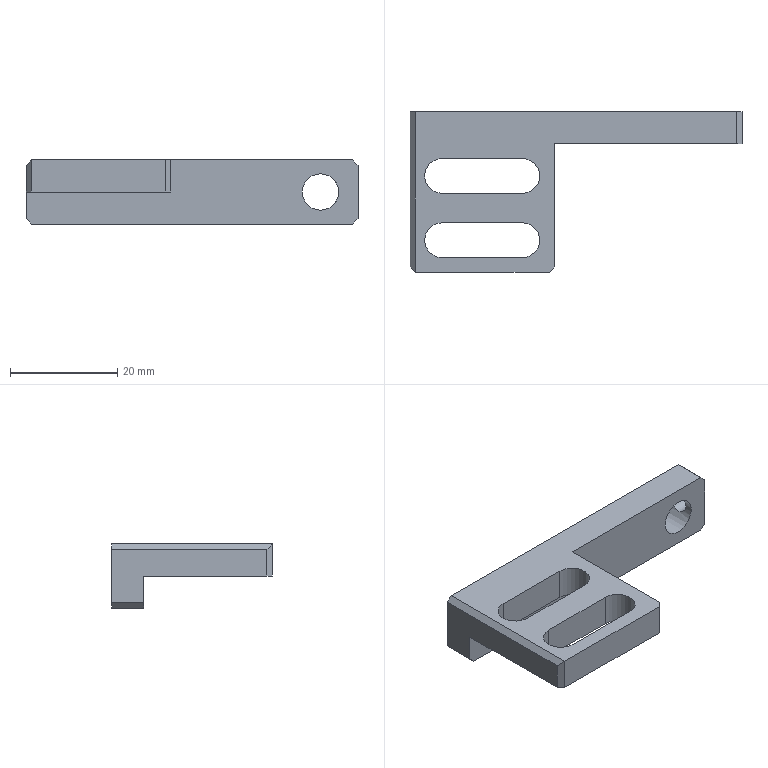NC program | NX | posted with a generic post | part box 62 x 30 x 12 mm
Whole program:
N10 G17 G21 G94 G90
(FLOOR_WALL_COPY , TOOL : D80)
N12 T19 M6
N14 G54
N16 G17 G0 G90 X-76. Y0. S6500 M3
N18 G43 Z30. H19
N20 Z5.
N22 G94 G1 Z2. F1500.
N24 X-73.
N26 X73.
N28 X76.
N30 Z5.
N32 G0 Z30.
N34 X-76.
N36 Z4.
N38 G1 Z1.
N40 X-73.
N42 X73.
N44 X76.
N46 Z4.
N48 G0 Z30.
N50 X-76.
N52 Z3.
N54 G1 Z0.
N56 X-73.
N58 X73.
N60 X76.
N62 Z3.
N64 G0 Z30.
N66 M5
(PLANAR_MILL_COPY_COPY_COPY_COPY_1 , TOOL : D6A45)
N68 T01 M6
N70 G54
N72 G17 G0 G90 X-0.866 Y16.4 S9500 M3
N74 G43 Z30. H1
N76 Z0.5
N78 G94 G1 Z-1. F1250.
N80 G3 X0. Y15.9 R1.
N82 G1 X31.
N84 G2 X31.9 Y15. R0.9
N86 G1 Y9.
N88 G2 X31. Y8.1 R0.9
N90 G1 X-3.1
N92 Y-14.
N94 G2 X-3.364 Y-14.636 R0.9
N96 G1 X-4.364 Y-15.636
N98 G2 X-5. Y-15.9 R0.9
N100 G1 X-30.
N102 G2 X-30.636 Y-15.636 R0.9
N104 G1 X-31.636 Y-14.636
N106 G2 X-31.9 Y-14. R0.9
N108 G1 Y15.
N110 G2 X-31. Y15.9 R0.9
N112 G1 X0.
N114 G3 X0.866 Y16.4 R1.
N116 G1 Z0.5
N118 G0 Z30.
N120 X-16.634 Y4.85
N122 Z0.5
N124 G1 Z-1.
N126 G3 X-17.5 Y5.35 R1.
N128 G1 X-25.
N130 G3 X-27.35 Y3. R2.35
N132 X-25. Y0.65 R2.35
N134 G1 X-10.
N136 G3 X-7.65 Y3. R2.35
N138 X-10. Y5.35 R2.35
N140 G1 X-17.5
N142 G3 X-18.366 Y4.85 R1.
N144 G1 Z0.5
N146 G0 Z30.
N148 Y-10.85
N150 Z0.5
N152 G1 Z-1.
N154 G3 X-17.5 Y-11.35 R1.
N156 G1 X-10.
N158 G3 X-7.65 Y-9. R2.35
N160 X-10. Y-6.65 R2.35
N162 G1 X-25.
N164 G3 X-27.35 Y-9. R2.35
N166 X-25. Y-11.35 R2.35
N168 G1 X-17.5
N170 G3 X-16.634 Y-10.85 R1.
N172 G1 Z0.5
N174 G0 Z30.
N176 M5
N178 M2